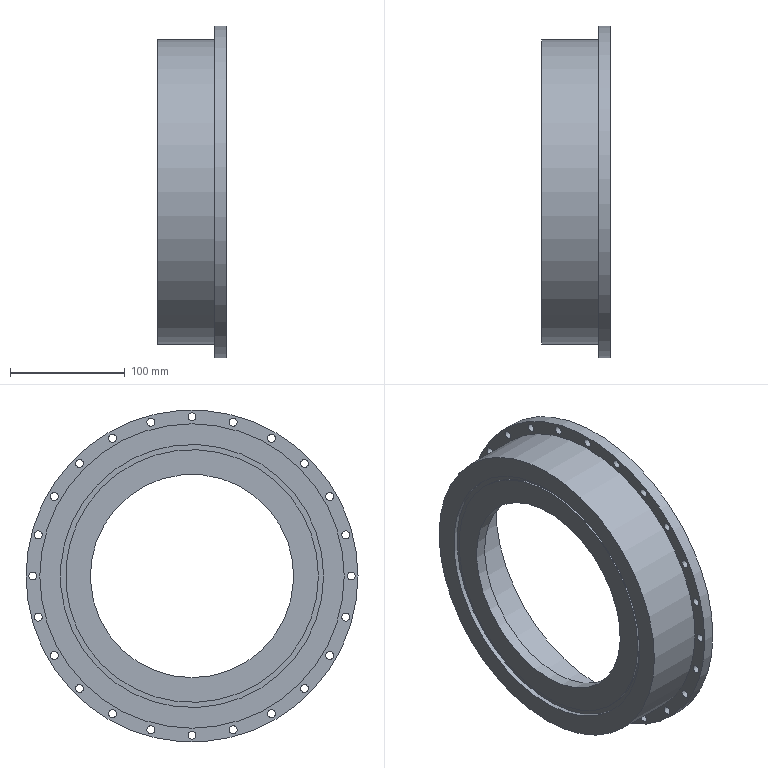Part | STEP file | Brake disc | 1 solid | 36 faces | box 60 x 289 x 289 mm | volume 806797 mm3 | cylinder 30 | plane 6 | commonest cylinder face diameters 7 x24 177 x1 220 x1 229 x1 245 x1 265 x1
STEP:
#1=CARTESIAN_POINT('',(-12.,0.,-132.5));
#2=VERTEX_POINT('',#1);
#3=CARTESIAN_POINT('',(-12.,0.,0.));
#4=DIRECTION('',(-1.,0.,0.));
#5=DIRECTION('',(0.,0.,-1.));
#6=AXIS2_PLACEMENT_3D('',#3,#4,#5);
#7=CIRCLE('',#6,132.5);
#8=EDGE_CURVE('',#2,#2,#7,.T.);
#9=ORIENTED_EDGE('',*,*,#8,.T.);
#10=EDGE_LOOP('',(#9));
#11=FACE_BOUND('',#10,.T.);
#12=CARTESIAN_POINT('',(-12.,-114.5,0.));
#13=VERTEX_POINT('',#12);
#14=CARTESIAN_POINT('',(-12.,0.,0.));
#15=DIRECTION('',(-1.,0.,0.));
#16=DIRECTION('',(0.,-1.,0.));
#17=AXIS2_PLACEMENT_3D('',#14,#15,#16);
#18=CIRCLE('',#17,114.5);
#19=EDGE_CURVE('',#13,#13,#18,.F.);
#20=ORIENTED_EDGE('',*,*,#19,.T.);
#21=EDGE_LOOP('',(#20));
#22=FACE_BOUND('',#21,.T.);
#23=CARTESIAN_POINT('',(-12.,0.,0.));
#24=DIRECTION('',(1.,0.,0.));
#25=DIRECTION('',(0.,1.,0.));
#26=AXIS2_PLACEMENT_3D('',#23,#24,#25);
#27=PLANE('',#26);
#28=ADVANCED_FACE('',(#11,#22),#27,.F.);
#29=CARTESIAN_POINT('',(-10.,-110.,0.));
#30=VERTEX_POINT('',#29);
#31=CARTESIAN_POINT('',(-10.,0.,0.));
#32=DIRECTION('',(-1.,0.,0.));
#33=DIRECTION('',(0.,-1.,0.));
#34=AXIS2_PLACEMENT_3D('',#31,#32,#33);
#35=CIRCLE('',#34,110.);
#36=EDGE_CURVE('',#30,#30,#35,.T.);
#37=ORIENTED_EDGE('',*,*,#36,.T.);
#38=EDGE_LOOP('',(#37));
#39=FACE_BOUND('',#38,.T.);
#40=CARTESIAN_POINT('',(-10.,0.,-88.5));
#41=VERTEX_POINT('',#40);
#42=CARTESIAN_POINT('',(-10.,0.,0.));
#43=DIRECTION('',(1.,0.,0.));
#44=DIRECTION('',(0.,0.,-1.));
#45=AXIS2_PLACEMENT_3D('',#42,#43,#44);
#46=CIRCLE('',#45,88.5);
#47=EDGE_CURVE('',#41,#41,#46,.T.);
#48=ORIENTED_EDGE('',*,*,#47,.T.);
#49=EDGE_LOOP('',(#48));
#50=FACE_BOUND('',#49,.T.);
#51=CARTESIAN_POINT('',(-10.,0.,0.));
#52=DIRECTION('',(1.,0.,0.));
#53=DIRECTION('',(0.,0.,-1.));
#54=AXIS2_PLACEMENT_3D('',#51,#52,#53);
#55=PLANE('',#54);
#56=ADVANCED_FACE('',(#39,#50),#55,.F.);
#57=CARTESIAN_POINT('',(-8.,-114.5,0.));
#58=VERTEX_POINT('',#57);
#59=CARTESIAN_POINT('',(-8.,0.,0.));
#60=DIRECTION('',(-1.,0.,0.));
#61=DIRECTION('',(0.,-1.,0.));
#62=AXIS2_PLACEMENT_3D('',#59,#60,#61);
#63=CIRCLE('',#62,114.5);
#64=EDGE_CURVE('',#58,#58,#63,.T.);
#65=ORIENTED_EDGE('',*,*,#64,.F.);
#66=EDGE_LOOP('',(#65));
#67=FACE_OUTER_BOUND('',#66,.T.);
#68=ORIENTED_EDGE('',*,*,#19,.F.);
#69=EDGE_LOOP('',(#68));
#70=FACE_OUTER_BOUND('',#69,.T.);
#71=CARTESIAN_POINT('',(-8.,0.,0.));
#72=DIRECTION('',(-1.,0.,0.));
#73=DIRECTION('',(0.,-1.,0.));
#74=AXIS2_PLACEMENT_3D('',#71,#72,#73);
#75=CYLINDRICAL_SURFACE('',#74,114.5);
#76=ADVANCED_FACE('',(#67,#70),#75,.F.);
#77=CARTESIAN_POINT('',(-8.,-110.,0.));
#78=VERTEX_POINT('',#77);
#79=CARTESIAN_POINT('',(-8.,0.,0.));
#80=DIRECTION('',(-1.,0.,0.));
#81=DIRECTION('',(0.,-1.,0.));
#82=AXIS2_PLACEMENT_3D('',#79,#80,#81);
#83=CIRCLE('',#82,110.);
#84=EDGE_CURVE('',#78,#78,#83,.T.);
#85=ORIENTED_EDGE('',*,*,#84,.T.);
#86=EDGE_LOOP('',(#85));
#87=FACE_OUTER_BOUND('',#86,.T.);
#88=ORIENTED_EDGE('',*,*,#36,.F.);
#89=EDGE_LOOP('',(#88));
#90=FACE_OUTER_BOUND('',#89,.T.);
#91=CARTESIAN_POINT('',(-8.,0.,0.));
#92=DIRECTION('',(-1.,0.,0.));
#93=DIRECTION('',(0.,-1.,0.));
#94=AXIS2_PLACEMENT_3D('',#91,#92,#93);
#95=CYLINDRICAL_SURFACE('',#94,110.);
#96=ADVANCED_FACE('',(#87,#90),#95,.T.);
#97=CARTESIAN_POINT('',(38.,0.,-132.5));
#98=VERTEX_POINT('',#97);
#99=CARTESIAN_POINT('',(38.,0.,0.));
#100=DIRECTION('',(-1.,0.,0.));
#101=DIRECTION('',(0.,0.,-1.));
#102=AXIS2_PLACEMENT_3D('',#99,#100,#101);
#103=CIRCLE('',#102,132.5);
#104=EDGE_CURVE('',#98,#98,#103,.F.);
#105=ORIENTED_EDGE('',*,*,#104,.F.);
#106=EDGE_LOOP('',(#105));
#107=FACE_OUTER_BOUND('',#106,.T.);
#108=ORIENTED_EDGE('',*,*,#8,.F.);
#109=EDGE_LOOP('',(#108));
#110=FACE_OUTER_BOUND('',#109,.T.);
#111=CARTESIAN_POINT('',(8.,0.,0.));
#112=DIRECTION('',(-1.,0.,0.));
#113=DIRECTION('',(0.,0.,-1.));
#114=AXIS2_PLACEMENT_3D('',#111,#112,#113);
#115=CYLINDRICAL_SURFACE('',#114,132.5);
#116=ADVANCED_FACE('',(#107,#110),#115,.T.);
#117=CARTESIAN_POINT('',(0.,0.,-88.5));
#118=VERTEX_POINT('',#117);
#119=CARTESIAN_POINT('',(0.,0.,0.));
#120=DIRECTION('',(1.,0.,0.));
#121=DIRECTION('',(0.,0.,-1.));
#122=AXIS2_PLACEMENT_3D('',#119,#120,#121);
#123=CIRCLE('',#122,88.5);
#124=EDGE_CURVE('',#118,#118,#123,.F.);
#125=ORIENTED_EDGE('',*,*,#124,.F.);
#126=EDGE_LOOP('',(#125));
#127=FACE_OUTER_BOUND('',#126,.T.);
#128=ORIENTED_EDGE('',*,*,#47,.F.);
#129=EDGE_LOOP('',(#128));
#130=FACE_OUTER_BOUND('',#129,.T.);
#131=CARTESIAN_POINT('',(-10.,0.,0.));
#132=DIRECTION('',(1.,0.,0.));
#133=DIRECTION('',(0.,0.,-1.));
#134=AXIS2_PLACEMENT_3D('',#131,#132,#133);
#135=CYLINDRICAL_SURFACE('',#134,88.5);
#136=ADVANCED_FACE('',(#127,#130),#135,.F.);
#137=ORIENTED_EDGE('',*,*,#64,.T.);
#138=EDGE_LOOP('',(#137));
#139=FACE_BOUND('',#138,.T.);
#140=ORIENTED_EDGE('',*,*,#84,.F.);
#141=EDGE_LOOP('',(#140));
#142=FACE_BOUND('',#141,.T.);
#143=CARTESIAN_POINT('',(-8.,0.,0.));
#144=DIRECTION('',(-1.,0.,0.));
#145=DIRECTION('',(0.,-1.,0.));
#146=AXIS2_PLACEMENT_3D('',#143,#144,#145);
#147=PLANE('',#146);
#148=ADVANCED_FACE('',(#139,#142),#147,.T.);
#149=CARTESIAN_POINT('',(38.,-144.5,0.));
#150=VERTEX_POINT('',#149);
#151=CARTESIAN_POINT('',(38.,0.,0.));
#152=DIRECTION('',(1.,0.,0.));
#153=DIRECTION('',(0.,-1.,0.));
#154=AXIS2_PLACEMENT_3D('',#151,#152,#153);
#155=CIRCLE('',#154,144.5);
#156=EDGE_CURVE('',#150,#150,#155,.T.);
#157=ORIENTED_EDGE('',*,*,#156,.F.);
#158=EDGE_LOOP('',(#157));
#159=FACE_BOUND('',#158,.T.);
#160=CARTESIAN_POINT('',(38.,137.161,36.752));
#161=VERTEX_POINT('',#160);
#162=CARTESIAN_POINT('',(38.,133.781,35.846));
#163=DIRECTION('',(1.,0.,0.));
#164=DIRECTION('',(0.,0.9659,0.2588));
#165=AXIS2_PLACEMENT_3D('',#162,#163,#164);
#166=CIRCLE('',#165,3.5);
#167=EDGE_CURVE('',#161,#161,#166,.T.);
#168=ORIENTED_EDGE('',*,*,#167,.T.);
#169=EDGE_LOOP('',(#168));
#170=FACE_BOUND('',#169,.T.);
#171=CARTESIAN_POINT('',(38.,122.976,71.));
#172=VERTEX_POINT('',#171);
#173=CARTESIAN_POINT('',(38.,119.945,69.25));
#174=DIRECTION('',(1.,0.,0.));
#175=DIRECTION('',(0.,0.866,0.5));
#176=AXIS2_PLACEMENT_3D('',#173,#174,#175);
#177=CIRCLE('',#176,3.5);
#178=EDGE_CURVE('',#172,#172,#177,.T.);
#179=ORIENTED_EDGE('',*,*,#178,.T.);
#180=EDGE_LOOP('',(#179));
#181=FACE_BOUND('',#180,.T.);
#182=CARTESIAN_POINT('',(38.,100.409,100.409));
#183=VERTEX_POINT('',#182);
#184=CARTESIAN_POINT('',(38.,97.934,97.934));
#185=DIRECTION('',(1.,0.,0.));
#186=DIRECTION('',(0.,0.7071,0.7071));
#187=AXIS2_PLACEMENT_3D('',#184,#185,#186);
#188=CIRCLE('',#187,3.5);
#189=EDGE_CURVE('',#183,#183,#188,.T.);
#190=ORIENTED_EDGE('',*,*,#189,.T.);
#191=EDGE_LOOP('',(#190));
#192=FACE_BOUND('',#191,.T.);
#193=CARTESIAN_POINT('',(38.,71.,122.976));
#194=VERTEX_POINT('',#193);
#195=CARTESIAN_POINT('',(38.,69.25,119.945));
#196=DIRECTION('',(1.,0.,0.));
#197=DIRECTION('',(0.,0.5,0.866));
#198=AXIS2_PLACEMENT_3D('',#195,#196,#197);
#199=CIRCLE('',#198,3.5);
#200=EDGE_CURVE('',#194,#194,#199,.T.);
#201=ORIENTED_EDGE('',*,*,#200,.T.);
#202=EDGE_LOOP('',(#201));
#203=FACE_BOUND('',#202,.T.);
#204=CARTESIAN_POINT('',(38.,36.752,137.161));
#205=VERTEX_POINT('',#204);
#206=CARTESIAN_POINT('',(38.,35.846,133.781));
#207=DIRECTION('',(1.,0.,0.));
#208=DIRECTION('',(0.,0.2588,0.9659));
#209=AXIS2_PLACEMENT_3D('',#206,#207,#208);
#210=CIRCLE('',#209,3.5);
#211=EDGE_CURVE('',#205,#205,#210,.T.);
#212=ORIENTED_EDGE('',*,*,#211,.T.);
#213=EDGE_LOOP('',(#212));
#214=FACE_BOUND('',#213,.T.);
#215=CARTESIAN_POINT('',(38.,0.,142.));
#216=VERTEX_POINT('',#215);
#217=CARTESIAN_POINT('',(38.,0.,138.5));
#218=DIRECTION('',(1.,0.,0.));
#219=DIRECTION('',(0.,0.,1.));
#220=AXIS2_PLACEMENT_3D('',#217,#218,#219);
#221=CIRCLE('',#220,3.5);
#222=EDGE_CURVE('',#216,#216,#221,.T.);
#223=ORIENTED_EDGE('',*,*,#222,.T.);
#224=EDGE_LOOP('',(#223));
#225=FACE_BOUND('',#224,.T.);
#226=CARTESIAN_POINT('',(38.,-36.752,137.161));
#227=VERTEX_POINT('',#226);
#228=CARTESIAN_POINT('',(38.,-35.846,133.781));
#229=DIRECTION('',(1.,0.,0.));
#230=DIRECTION('',(0.,-0.2588,0.9659));
#231=AXIS2_PLACEMENT_3D('',#228,#229,#230);
#232=CIRCLE('',#231,3.5);
#233=EDGE_CURVE('',#227,#227,#232,.T.);
#234=ORIENTED_EDGE('',*,*,#233,.T.);
#235=EDGE_LOOP('',(#234));
#236=FACE_BOUND('',#235,.T.);
#237=CARTESIAN_POINT('',(38.,-71.,122.976));
#238=VERTEX_POINT('',#237);
#239=CARTESIAN_POINT('',(38.,-69.25,119.945));
#240=DIRECTION('',(1.,0.,0.));
#241=DIRECTION('',(0.,-0.5,0.866));
#242=AXIS2_PLACEMENT_3D('',#239,#240,#241);
#243=CIRCLE('',#242,3.5);
#244=EDGE_CURVE('',#238,#238,#243,.T.);
#245=ORIENTED_EDGE('',*,*,#244,.T.);
#246=EDGE_LOOP('',(#245));
#247=FACE_BOUND('',#246,.T.);
#248=CARTESIAN_POINT('',(38.,-100.409,100.409));
#249=VERTEX_POINT('',#248);
#250=CARTESIAN_POINT('',(38.,-97.934,97.934));
#251=DIRECTION('',(1.,0.,0.));
#252=DIRECTION('',(0.,-0.7071,0.7071));
#253=AXIS2_PLACEMENT_3D('',#250,#251,#252);
#254=CIRCLE('',#253,3.5);
#255=EDGE_CURVE('',#249,#249,#254,.T.);
#256=ORIENTED_EDGE('',*,*,#255,.T.);
#257=EDGE_LOOP('',(#256));
#258=FACE_BOUND('',#257,.T.);
#259=CARTESIAN_POINT('',(38.,-122.976,71.));
#260=VERTEX_POINT('',#259);
#261=CARTESIAN_POINT('',(38.,-119.945,69.25));
#262=DIRECTION('',(1.,0.,0.));
#263=DIRECTION('',(0.,-0.866,0.5));
#264=AXIS2_PLACEMENT_3D('',#261,#262,#263);
#265=CIRCLE('',#264,3.5);
#266=EDGE_CURVE('',#260,#260,#265,.T.);
#267=ORIENTED_EDGE('',*,*,#266,.T.);
#268=EDGE_LOOP('',(#267));
#269=FACE_BOUND('',#268,.T.);
#270=CARTESIAN_POINT('',(38.,-137.161,36.752));
#271=VERTEX_POINT('',#270);
#272=CARTESIAN_POINT('',(38.,-133.781,35.846));
#273=DIRECTION('',(1.,0.,0.));
#274=DIRECTION('',(0.,-0.9659,0.2588));
#275=AXIS2_PLACEMENT_3D('',#272,#273,#274);
#276=CIRCLE('',#275,3.5);
#277=EDGE_CURVE('',#271,#271,#276,.T.);
#278=ORIENTED_EDGE('',*,*,#277,.T.);
#279=EDGE_LOOP('',(#278));
#280=FACE_BOUND('',#279,.T.);
#281=CARTESIAN_POINT('',(38.,-142.,0.));
#282=VERTEX_POINT('',#281);
#283=CARTESIAN_POINT('',(38.,-138.5,0.));
#284=DIRECTION('',(1.,0.,0.));
#285=DIRECTION('',(0.,-1.,0.));
#286=AXIS2_PLACEMENT_3D('',#283,#284,#285);
#287=CIRCLE('',#286,3.5);
#288=EDGE_CURVE('',#282,#282,#287,.T.);
#289=ORIENTED_EDGE('',*,*,#288,.T.);
#290=EDGE_LOOP('',(#289));
#291=FACE_BOUND('',#290,.T.);
#292=CARTESIAN_POINT('',(38.,-137.161,-36.752));
#293=VERTEX_POINT('',#292);
#294=CARTESIAN_POINT('',(38.,-133.781,-35.846));
#295=DIRECTION('',(1.,0.,0.));
#296=DIRECTION('',(0.,-0.9659,-0.2588));
#297=AXIS2_PLACEMENT_3D('',#294,#295,#296);
#298=CIRCLE('',#297,3.5);
#299=EDGE_CURVE('',#293,#293,#298,.T.);
#300=ORIENTED_EDGE('',*,*,#299,.T.);
#301=EDGE_LOOP('',(#300));
#302=FACE_BOUND('',#301,.T.);
#303=CARTESIAN_POINT('',(38.,-122.976,-71.));
#304=VERTEX_POINT('',#303);
#305=CARTESIAN_POINT('',(38.,-119.945,-69.25));
#306=DIRECTION('',(1.,0.,0.));
#307=DIRECTION('',(0.,-0.866,-0.5));
#308=AXIS2_PLACEMENT_3D('',#305,#306,#307);
#309=CIRCLE('',#308,3.5);
#310=EDGE_CURVE('',#304,#304,#309,.T.);
#311=ORIENTED_EDGE('',*,*,#310,.T.);
#312=EDGE_LOOP('',(#311));
#313=FACE_BOUND('',#312,.T.);
#314=CARTESIAN_POINT('',(38.,-100.409,-100.409));
#315=VERTEX_POINT('',#314);
#316=CARTESIAN_POINT('',(38.,-97.934,-97.934));
#317=DIRECTION('',(1.,0.,0.));
#318=DIRECTION('',(0.,-0.7071,-0.7071));
#319=AXIS2_PLACEMENT_3D('',#316,#317,#318);
#320=CIRCLE('',#319,3.5);
#321=EDGE_CURVE('',#315,#315,#320,.T.);
#322=ORIENTED_EDGE('',*,*,#321,.T.);
#323=EDGE_LOOP('',(#322));
#324=FACE_BOUND('',#323,.T.);
#325=CARTESIAN_POINT('',(38.,-71.,-122.976));
#326=VERTEX_POINT('',#325);
#327=CARTESIAN_POINT('',(38.,-69.25,-119.945));
#328=DIRECTION('',(1.,0.,0.));
#329=DIRECTION('',(0.,-0.5,-0.866));
#330=AXIS2_PLACEMENT_3D('',#327,#328,#329);
#331=CIRCLE('',#330,3.5);
#332=EDGE_CURVE('',#326,#326,#331,.T.);
#333=ORIENTED_EDGE('',*,*,#332,.T.);
#334=EDGE_LOOP('',(#333));
#335=FACE_BOUND('',#334,.T.);
#336=CARTESIAN_POINT('',(38.,-36.752,-137.161));
#337=VERTEX_POINT('',#336);
#338=CARTESIAN_POINT('',(38.,-35.846,-133.781));
#339=DIRECTION('',(1.,0.,0.));
#340=DIRECTION('',(0.,-0.2588,-0.9659));
#341=AXIS2_PLACEMENT_3D('',#338,#339,#340);
#342=CIRCLE('',#341,3.5);
#343=EDGE_CURVE('',#337,#337,#342,.T.);
#344=ORIENTED_EDGE('',*,*,#343,.T.);
#345=EDGE_LOOP('',(#344));
#346=FACE_BOUND('',#345,.T.);
#347=CARTESIAN_POINT('',(38.,0.,-142.));
#348=VERTEX_POINT('',#347);
#349=CARTESIAN_POINT('',(38.,0.,-138.5));
#350=DIRECTION('',(1.,0.,0.));
#351=DIRECTION('',(0.,0.,-1.));
#352=AXIS2_PLACEMENT_3D('',#349,#350,#351);
#353=CIRCLE('',#352,3.5);
#354=EDGE_CURVE('',#348,#348,#353,.T.);
#355=ORIENTED_EDGE('',*,*,#354,.T.);
#356=EDGE_LOOP('',(#355));
#357=FACE_BOUND('',#356,.T.);
#358=CARTESIAN_POINT('',(38.,36.752,-137.161));
#359=VERTEX_POINT('',#358);
#360=CARTESIAN_POINT('',(38.,35.846,-133.781));
#361=DIRECTION('',(1.,0.,0.));
#362=DIRECTION('',(0.,0.2588,-0.9659));
#363=AXIS2_PLACEMENT_3D('',#360,#361,#362);
#364=CIRCLE('',#363,3.5);
#365=EDGE_CURVE('',#359,#359,#364,.T.);
#366=ORIENTED_EDGE('',*,*,#365,.T.);
#367=EDGE_LOOP('',(#366));
#368=FACE_BOUND('',#367,.T.);
#369=CARTESIAN_POINT('',(38.,71.,-122.976));
#370=VERTEX_POINT('',#369);
#371=CARTESIAN_POINT('',(38.,69.25,-119.945));
#372=DIRECTION('',(1.,0.,0.));
#373=DIRECTION('',(0.,0.5,-0.866));
#374=AXIS2_PLACEMENT_3D('',#371,#372,#373);
#375=CIRCLE('',#374,3.5);
#376=EDGE_CURVE('',#370,#370,#375,.T.);
#377=ORIENTED_EDGE('',*,*,#376,.T.);
#378=EDGE_LOOP('',(#377));
#379=FACE_BOUND('',#378,.T.);
#380=CARTESIAN_POINT('',(38.,100.409,-100.409));
#381=VERTEX_POINT('',#380);
#382=CARTESIAN_POINT('',(38.,97.934,-97.934));
#383=DIRECTION('',(1.,0.,0.));
#384=DIRECTION('',(0.,0.7071,-0.7071));
#385=AXIS2_PLACEMENT_3D('',#382,#383,#384);
#386=CIRCLE('',#385,3.5);
#387=EDGE_CURVE('',#381,#381,#386,.T.);
#388=ORIENTED_EDGE('',*,*,#387,.T.);
#389=EDGE_LOOP('',(#388));
#390=FACE_BOUND('',#389,.T.);
#391=CARTESIAN_POINT('',(38.,122.976,-71.));
#392=VERTEX_POINT('',#391);
#393=CARTESIAN_POINT('',(38.,119.945,-69.25));
#394=DIRECTION('',(1.,0.,0.));
#395=DIRECTION('',(0.,0.866,-0.5));
#396=AXIS2_PLACEMENT_3D('',#393,#394,#395);
#397=CIRCLE('',#396,3.5);
#398=EDGE_CURVE('',#392,#392,#397,.T.);
#399=ORIENTED_EDGE('',*,*,#398,.T.);
#400=EDGE_LOOP('',(#399));
#401=FACE_BOUND('',#400,.T.);
#402=CARTESIAN_POINT('',(38.,137.161,-36.752));
#403=VERTEX_POINT('',#402);
#404=CARTESIAN_POINT('',(38.,133.781,-35.846));
#405=DIRECTION('',(1.,0.,0.));
#406=DIRECTION('',(0.,0.9659,-0.2588));
#407=AXIS2_PLACEMENT_3D('',#404,#405,#406);
#408=CIRCLE('',#407,3.5);
#409=EDGE_CURVE('',#403,#403,#408,.T.);
#410=ORIENTED_EDGE('',*,*,#409,.T.);
#411=EDGE_LOOP('',(#410));
#412=FACE_BOUND('',#411,.T.);
#413=ORIENTED_EDGE('',*,*,#104,.T.);
#414=EDGE_LOOP('',(#413));
#415=FACE_BOUND('',#414,.T.);
#416=CARTESIAN_POINT('',(38.,142.,0.));
#417=VERTEX_POINT('',#416);
#418=CARTESIAN_POINT('',(38.,138.5,0.));
#419=DIRECTION('',(1.,0.,0.));
#420=DIRECTION('',(0.,1.,0.));
#421=AXIS2_PLACEMENT_3D('',#418,#419,#420);
#422=CIRCLE('',#421,3.5);
#423=EDGE_CURVE('',#417,#417,#422,.T.);
#424=ORIENTED_EDGE('',*,*,#423,.T.);
#425=EDGE_LOOP('',(#424));
#426=FACE_BOUND('',#425,.T.);
#427=CARTESIAN_POINT('',(38.,0.,0.));
#428=DIRECTION('',(1.,0.,0.));
#429=DIRECTION('',(0.,-1.,0.));
#430=AXIS2_PLACEMENT_3D('',#427,#428,#429);
#431=PLANE('',#430);
#432=ADVANCED_FACE('',(#159,#170,#181,#192,#203,#214,#225,#236,#247,#258,#269,#280,#291,#302,#313,#324,#335,#346,#357,#368,#379,#390,#401,#412,#415,#426),#431,.F.);
#433=CARTESIAN_POINT('',(0.,0.,-122.5));
#434=VERTEX_POINT('',#433);
#435=CARTESIAN_POINT('',(0.,0.,0.));
#436=DIRECTION('',(1.,0.,0.));
#437=DIRECTION('',(0.,0.,-1.));
#438=AXIS2_PLACEMENT_3D('',#435,#436,#437);
#439=CIRCLE('',#438,122.5);
#440=EDGE_CURVE('',#434,#434,#439,.F.);
#441=ORIENTED_EDGE('',*,*,#440,.F.);
#442=EDGE_LOOP('',(#441));
#443=FACE_BOUND('',#442,.T.);
#444=ORIENTED_EDGE('',*,*,#124,.T.);
#445=EDGE_LOOP('',(#444));
#446=FACE_BOUND('',#445,.T.);
#447=CARTESIAN_POINT('',(0.,0.,0.));
#448=DIRECTION('',(1.,0.,0.));
#449=DIRECTION('',(0.,0.,-1.));
#450=AXIS2_PLACEMENT_3D('',#447,#448,#449);
#451=PLANE('',#450);
#452=ADVANCED_FACE('',(#443,#446),#451,.T.);
#453=CARTESIAN_POINT('',(48.,-144.5,0.));
#454=VERTEX_POINT('',#453);
#455=CARTESIAN_POINT('',(48.,0.,0.));
#456=DIRECTION('',(1.,0.,0.));
#457=DIRECTION('',(0.,-1.,0.));
#458=AXIS2_PLACEMENT_3D('',#455,#456,#457);
#459=CIRCLE('',#458,144.5);
#460=EDGE_CURVE('',#454,#454,#459,.T.);
#461=ORIENTED_EDGE('',*,*,#460,.F.);
#462=EDGE_LOOP('',(#461));
#463=FACE_OUTER_BOUND('',#462,.T.);
#464=ORIENTED_EDGE('',*,*,#156,.T.);
#465=EDGE_LOOP('',(#464));
#466=FACE_OUTER_BOUND('',#465,.T.);
#467=CARTESIAN_POINT('',(38.,0.,0.));
#468=DIRECTION('',(1.,0.,0.));
#469=DIRECTION('',(0.,-1.,0.));
#470=AXIS2_PLACEMENT_3D('',#467,#468,#469);
#471=CYLINDRICAL_SURFACE('',#470,144.5);
#472=ADVANCED_FACE('',(#463,#466),#471,.T.);
#473=CARTESIAN_POINT('',(48.,137.161,36.752));
#474=VERTEX_POINT('',#473);
#475=CARTESIAN_POINT('',(48.,133.781,35.846));
#476=DIRECTION('',(1.,0.,0.));
#477=DIRECTION('',(0.,0.9659,0.2588));
#478=AXIS2_PLACEMENT_3D('',#475,#476,#477);
#479=CIRCLE('',#478,3.5);
#480=EDGE_CURVE('',#474,#474,#479,.F.);
#481=ORIENTED_EDGE('',*,*,#480,.F.);
#482=EDGE_LOOP('',(#481));
#483=FACE_OUTER_BOUND('',#482,.T.);
#484=ORIENTED_EDGE('',*,*,#167,.F.);
#485=EDGE_LOOP('',(#484));
#486=FACE_OUTER_BOUND('',#485,.T.);
#487=CARTESIAN_POINT('',(8.,133.781,35.846));
#488=DIRECTION('',(1.,0.,0.));
#489=DIRECTION('',(0.,0.9659,0.2588));
#490=AXIS2_PLACEMENT_3D('',#487,#488,#489);
#491=CYLINDRICAL_SURFACE('',#490,3.5);
#492=ADVANCED_FACE('',(#483,#486),#491,.F.);
#493=CARTESIAN_POINT('',(48.,122.976,71.));
#494=VERTEX_POINT('',#493);
#495=CARTESIAN_POINT('',(48.,119.945,69.25));
#496=DIRECTION('',(1.,0.,0.));
#497=DIRECTION('',(0.,0.866,0.5));
#498=AXIS2_PLACEMENT_3D('',#495,#496,#497);
#499=CIRCLE('',#498,3.5);
#500=EDGE_CURVE('',#494,#494,#499,.F.);
#501=ORIENTED_EDGE('',*,*,#500,.F.);
#502=EDGE_LOOP('',(#501));
#503=FACE_OUTER_BOUND('',#502,.T.);
#504=ORIENTED_EDGE('',*,*,#178,.F.);
#505=EDGE_LOOP('',(#504));
#506=FACE_OUTER_BOUND('',#505,.T.);
#507=CARTESIAN_POINT('',(8.,119.945,69.25));
#508=DIRECTION('',(1.,0.,0.));
#509=DIRECTION('',(0.,0.866,0.5));
#510=AXIS2_PLACEMENT_3D('',#507,#508,#509);
#511=CYLINDRICAL_SURFACE('',#510,3.5);
#512=ADVANCED_FACE('',(#503,#506),#511,.F.);
#513=CARTESIAN_POINT('',(48.,100.409,100.409));
#514=VERTEX_POINT('',#513);
#515=CARTESIAN_POINT('',(48.,97.934,97.934));
#516=DIRECTION('',(1.,0.,0.));
#517=DIRECTION('',(0.,0.7071,0.7071));
#518=AXIS2_PLACEMENT_3D('',#515,#516,#517);
#519=CIRCLE('',#518,3.5);
#520=EDGE_CURVE('',#514,#514,#519,.F.);
#521=ORIENTED_EDGE('',*,*,#520,.F.);
#522=EDGE_LOOP('',(#521));
#523=FACE_OUTER_BOUND('',#522,.T.);
#524=ORIENTED_EDGE('',*,*,#189,.F.);
#525=EDGE_LOOP('',(#524));
#526=FACE_OUTER_BOUND('',#525,.T.);
#527=CARTESIAN_POINT('',(8.,97.934,97.934));
#528=DIRECTION('',(1.,0.,0.));
#529=DIRECTION('',(0.,0.7071,0.7071));
#530=AXIS2_PLACEMENT_3D('',#527,#528,#529);
#531=CYLINDRICAL_SURFACE('',#530,3.5);
#532=ADVANCED_FACE('',(#523,#526),#531,.F.);
#533=CARTESIAN_POINT('',(48.,71.,122.976));
#534=VERTEX_POINT('',#533);
#535=CARTESIAN_POINT('',(48.,69.25,119.945));
#536=DIRECTION('',(1.,0.,0.));
#537=DIRECTION('',(0.,0.5,0.866));
#538=AXIS2_PLACEMENT_3D('',#535,#536,#537);
#539=CIRCLE('',#538,3.5);
#540=EDGE_CURVE('',#534,#534,#539,.F.);
#541=ORIENTED_EDGE('',*,*,#540,.F.);
#542=EDGE_LOOP('',(#541));
#543=FACE_OUTER_BOUND('',#542,.T.);
#544=ORIENTED_EDGE('',*,*,#200,.F.);
#545=EDGE_LOOP('',(#544));
#546=FACE_OUTER_BOUND('',#545,.T.);
#547=CARTESIAN_POINT('',(8.,69.25,119.945));
#548=DIRECTION('',(1.,0.,0.));
#549=DIRECTION('',(0.,0.5,0.866));
#550=AXIS2_PLACEMENT_3D('',#547,#548,#549);
#551=CYLINDRICAL_SURFACE('',#550,3.5);
#552=ADVANCED_FACE('',(#543,#546),#551,.F.);
#553=CARTESIAN_POINT('',(48.,36.752,137.161));
#554=VERTEX_POINT('',#553);
#555=CARTESIAN_POINT('',(48.,35.846,133.781));
#556=DIRECTION('',(1.,0.,0.));
#557=DIRECTION('',(0.,0.2588,0.9659));
#558=AXIS2_PLACEMENT_3D('',#555,#556,#557);
#559=CIRCLE('',#558,3.5);
#560=EDGE_CURVE('',#554,#554,#559,.F.);
#561=ORIENTED_EDGE('',*,*,#560,.F.);
#562=EDGE_LOOP('',(#561));
#563=FACE_OUTER_BOUND('',#562,.T.);
#564=ORIENTED_EDGE('',*,*,#211,.F.);
#565=EDGE_LOOP('',(#564));
#566=FACE_OUTER_BOUND('',#565,.T.);
#567=CARTESIAN_POINT('',(8.,35.846,133.781));
#568=DIRECTION('',(1.,0.,0.));
#569=DIRECTION('',(0.,0.2588,0.9659));
#570=AXIS2_PLACEMENT_3D('',#567,#568,#569);
#571=CYLINDRICAL_SURFACE('',#570,3.5);
#572=ADVANCED_FACE('',(#563,#566),#571,.F.);
#573=CARTESIAN_POINT('',(48.,0.,142.));
#574=VERTEX_POINT('',#573);
#575=CARTESIAN_POINT('',(48.,0.,138.5));
#576=DIRECTION('',(1.,0.,0.));
#577=DIRECTION('',(0.,0.,1.));
#578=AXIS2_PLACEMENT_3D('',#575,#576,#577);
#579=CIRCLE('',#578,3.5);
#580=EDGE_CURVE('',#574,#574,#579,.F.);
#581=ORIENTED_EDGE('',*,*,#580,.F.);
#582=EDGE_LOOP('',(#581));
#583=FACE_OUTER_BOUND('',#582,.T.);
#584=ORIENTED_EDGE('',*,*,#222,.F.);
#585=EDGE_LOOP('',(#584));
#586=FACE_OUTER_BOUND('',#585,.T.);
#587=CARTESIAN_POINT('',(8.,0.,138.5));
#588=DIRECTION('',(1.,0.,0.));
#589=DIRECTION('',(0.,0.,1.));
#590=AXIS2_PLACEMENT_3D('',#587,#588,#589);
#591=CYLINDRICAL_SURFACE('',#590,3.5);
#592=ADVANCED_FACE('',(#583,#586),#591,.F.);
#593=CARTESIAN_POINT('',(48.,-36.752,137.161));
#594=VERTEX_POINT('',#593);
#595=CARTESIAN_POINT('',(48.,-35.846,133.781));
#596=DIRECTION('',(1.,0.,0.));
#597=DIRECTION('',(0.,-0.2588,0.9659));
#598=AXIS2_PLACEMENT_3D('',#595,#596,#597);
#599=CIRCLE('',#598,3.5);
#600=EDGE_CURVE('',#594,#594,#599,.F.);
#601=ORIENTED_EDGE('',*,*,#600,.F.);
#602=EDGE_LOOP('',(#601));
#603=FACE_OUTER_BOUND('',#602,.T.);
#604=ORIENTED_EDGE('',*,*,#233,.F.);
#605=EDGE_LOOP('',(#604));
#606=FACE_OUTER_BOUND('',#605,.T.);
#607=CARTESIAN_POINT('',(8.,-35.846,133.781));
#608=DIRECTION('',(1.,0.,0.));
#609=DIRECTION('',(0.,-0.2588,0.9659));
#610=AXIS2_PLACEMENT_3D('',#607,#608,#609);
#611=CYLINDRICAL_SURFACE('',#610,3.5);
#612=ADVANCED_FACE('',(#603,#606),#611,.F.);
#613=CARTESIAN_POINT('',(48.,-71.,122.976));
#614=VERTEX_POINT('',#613);
#615=CARTESIAN_POINT('',(48.,-69.25,119.945));
#616=DIRECTION('',(1.,0.,0.));
#617=DIRECTION('',(0.,-0.5,0.866));
#618=AXIS2_PLACEMENT_3D('',#615,#616,#617);
#619=CIRCLE('',#618,3.5);
#620=EDGE_CURVE('',#614,#614,#619,.F.);
#621=ORIENTED_EDGE('',*,*,#620,.F.);
#622=EDGE_LOOP('',(#621));
#623=FACE_OUTER_BOUND('',#622,.T.);
#624=ORIENTED_EDGE('',*,*,#244,.F.);
#625=EDGE_LOOP('',(#624));
#626=FACE_OUTER_BOUND('',#625,.T.);
#627=CARTESIAN_POINT('',(8.,-69.25,119.945));
#628=DIRECTION('',(1.,0.,0.));
#629=DIRECTION('',(0.,-0.5,0.866));
#630=AXIS2_PLACEMENT_3D('',#627,#628,#629);
#631=CYLINDRICAL_SURFACE('',#630,3.5);
#632=ADVANCED_FACE('',(#623,#626),#631,.F.);
#633=CARTESIAN_POINT('',(48.,-100.409,100.409));
#634=VERTEX_POINT('',#633);
#635=CARTESIAN_POINT('',(48.,-97.934,97.934));
#636=DIRECTION('',(1.,0.,0.));
#637=DIRECTION('',(0.,-0.7071,0.7071));
#638=AXIS2_PLACEMENT_3D('',#635,#636,#637);
#639=CIRCLE('',#638,3.5);
#640=EDGE_CURVE('',#634,#634,#639,.F.);
#641=ORIENTED_EDGE('',*,*,#640,.F.);
#642=EDGE_LOOP('',(#641));
#643=FACE_OUTER_BOUND('',#642,.T.);
#644=ORIENTED_EDGE('',*,*,#255,.F.);
#645=EDGE_LOOP('',(#644));
#646=FACE_OUTER_BOUND('',#645,.T.);
#647=CARTESIAN_POINT('',(8.,-97.934,97.934));
#648=DIRECTION('',(1.,0.,0.));
#649=DIRECTION('',(0.,-0.7071,0.7071));
#650=AXIS2_PLACEMENT_3D('',#647,#648,#649);
#651=CYLINDRICAL_SURFACE('',#650,3.5);
#652=ADVANCED_FACE('',(#643,#646),#651,.F.);
#653=CARTESIAN_POINT('',(48.,-122.976,71.));
#654=VERTEX_POINT('',#653);
#655=CARTESIAN_POINT('',(48.,-119.945,69.25));
#656=DIRECTION('',(1.,0.,0.));
#657=DIRECTION('',(0.,-0.866,0.5));
#658=AXIS2_PLACEMENT_3D('',#655,#656,#657);
#659=CIRCLE('',#658,3.5);
#660=EDGE_CURVE('',#654,#654,#659,.F.);
#661=ORIENTED_EDGE('',*,*,#660,.F.);
#662=EDGE_LOOP('',(#661));
#663=FACE_OUTER_BOUND('',#662,.T.);
#664=ORIENTED_EDGE('',*,*,#266,.F.);
#665=EDGE_LOOP('',(#664));
#666=FACE_OUTER_BOUND('',#665,.T.);
#667=CARTESIAN_POINT('',(8.,-119.945,69.25));
#668=DIRECTION('',(1.,0.,0.));
#669=DIRECTION('',(0.,-0.866,0.5));
#670=AXIS2_PLACEMENT_3D('',#667,#668,#669);
#671=CYLINDRICAL_SURFACE('',#670,3.5);
#672=ADVANCED_FACE('',(#663,#666),#671,.F.);
#673=CARTESIAN_POINT('',(48.,-137.161,36.752));
#674=VERTEX_POINT('',#673);
#675=CARTESIAN_POINT('',(48.,-133.781,35.846));
#676=DIRECTION('',(1.,0.,0.));
#677=DIRECTION('',(0.,-0.9659,0.2588));
#678=AXIS2_PLACEMENT_3D('',#675,#676,#677);
#679=CIRCLE('',#678,3.5);
#680=EDGE_CURVE('',#674,#674,#679,.F.);
#681=ORIENTED_EDGE('',*,*,#680,.F.);
#682=EDGE_LOOP('',(#681));
#683=FACE_OUTER_BOUND('',#682,.T.);
#684=ORIENTED_EDGE('',*,*,#277,.F.);
#685=EDGE_LOOP('',(#684));
#686=FACE_OUTER_BOUND('',#685,.T.);
#687=CARTESIAN_POINT('',(8.,-133.781,35.846));
#688=DIRECTION('',(1.,0.,0.));
#689=DIRECTION('',(0.,-0.9659,0.2588));
#690=AXIS2_PLACEMENT_3D('',#687,#688,#689);
#691=CYLINDRICAL_SURFACE('',#690,3.5);
#692=ADVANCED_FACE('',(#683,#686),#691,.F.);
#693=CARTESIAN_POINT('',(48.,-142.,0.));
#694=VERTEX_POINT('',#693);
#695=CARTESIAN_POINT('',(48.,-138.5,0.));
#696=DIRECTION('',(1.,0.,0.));
#697=DIRECTION('',(0.,-1.,0.));
#698=AXIS2_PLACEMENT_3D('',#695,#696,#697);
#699=CIRCLE('',#698,3.5);
#700=EDGE_CURVE('',#694,#694,#699,.F.);
#701=ORIENTED_EDGE('',*,*,#700,.F.);
#702=EDGE_LOOP('',(#701));
#703=FACE_OUTER_BOUND('',#702,.T.);
#704=ORIENTED_EDGE('',*,*,#288,.F.);
#705=EDGE_LOOP('',(#704));
#706=FACE_OUTER_BOUND('',#705,.T.);
#707=CARTESIAN_POINT('',(8.,-138.5,0.));
#708=DIRECTION('',(1.,0.,0.));
#709=DIRECTION('',(0.,-1.,0.));
#710=AXIS2_PLACEMENT_3D('',#707,#708,#709);
#711=CYLINDRICAL_SURFACE('',#710,3.5);
#712=ADVANCED_FACE('',(#703,#706),#711,.F.);
#713=CARTESIAN_POINT('',(48.,-137.161,-36.752));
#714=VERTEX_POINT('',#713);
#715=CARTESIAN_POINT('',(48.,-133.781,-35.846));
#716=DIRECTION('',(1.,0.,0.));
#717=DIRECTION('',(0.,-0.9659,-0.2588));
#718=AXIS2_PLACEMENT_3D('',#715,#716,#717);
#719=CIRCLE('',#718,3.5);
#720=EDGE_CURVE('',#714,#714,#719,.F.);
#721=ORIENTED_EDGE('',*,*,#720,.F.);
#722=EDGE_LOOP('',(#721));
#723=FACE_OUTER_BOUND('',#722,.T.);
#724=ORIENTED_EDGE('',*,*,#299,.F.);
#725=EDGE_LOOP('',(#724));
#726=FACE_OUTER_BOUND('',#725,.T.);
#727=CARTESIAN_POINT('',(8.,-133.781,-35.846));
#728=DIRECTION('',(1.,0.,0.));
#729=DIRECTION('',(0.,-0.9659,-0.2588));
#730=AXIS2_PLACEMENT_3D('',#727,#728,#729);
#731=CYLINDRICAL_SURFACE('',#730,3.5);
#732=ADVANCED_FACE('',(#723,#726),#731,.F.);
#733=CARTESIAN_POINT('',(48.,-122.976,-71.));
#734=VERTEX_POINT('',#733);
#735=CARTESIAN_POINT('',(48.,-119.945,-69.25));
#736=DIRECTION('',(1.,0.,0.));
#737=DIRECTION('',(0.,-0.866,-0.5));
#738=AXIS2_PLACEMENT_3D('',#735,#736,#737);
#739=CIRCLE('',#738,3.5);
#740=EDGE_CURVE('',#734,#734,#739,.F.);
#741=ORIENTED_EDGE('',*,*,#740,.F.);
#742=EDGE_LOOP('',(#741));
#743=FACE_OUTER_BOUND('',#742,.T.);
#744=ORIENTED_EDGE('',*,*,#310,.F.);
#745=EDGE_LOOP('',(#744));
#746=FACE_OUTER_BOUND('',#745,.T.);
#747=CARTESIAN_POINT('',(8.,-119.945,-69.25));
#748=DIRECTION('',(1.,0.,0.));
#749=DIRECTION('',(0.,-0.866,-0.5));
#750=AXIS2_PLACEMENT_3D('',#747,#748,#749);
#751=CYLINDRICAL_SURFACE('',#750,3.5);
#752=ADVANCED_FACE('',(#743,#746),#751,.F.);
#753=CARTESIAN_POINT('',(48.,-100.409,-100.409));
#754=VERTEX_POINT('',#753);
#755=CARTESIAN_POINT('',(48.,-97.934,-97.934));
#756=DIRECTION('',(1.,0.,0.));
#757=DIRECTION('',(0.,-0.7071,-0.7071));
#758=AXIS2_PLACEMENT_3D('',#755,#756,#757);
#759=CIRCLE('',#758,3.5);
#760=EDGE_CURVE('',#754,#754,#759,.F.);
#761=ORIENTED_EDGE('',*,*,#760,.F.);
#762=EDGE_LOOP('',(#761));
#763=FACE_OUTER_BOUND('',#762,.T.);
#764=ORIENTED_EDGE('',*,*,#321,.F.);
#765=EDGE_LOOP('',(#764));
#766=FACE_OUTER_BOUND('',#765,.T.);
#767=CARTESIAN_POINT('',(8.,-97.934,-97.934));
#768=DIRECTION('',(1.,0.,0.));
#769=DIRECTION('',(0.,-0.7071,-0.7071));
#770=AXIS2_PLACEMENT_3D('',#767,#768,#769);
#771=CYLINDRICAL_SURFACE('',#770,3.5);
#772=ADVANCED_FACE('',(#763,#766),#771,.F.);
#773=CARTESIAN_POINT('',(48.,-71.,-122.976));
#774=VERTEX_POINT('',#773);
#775=CARTESIAN_POINT('',(48.,-69.25,-119.945));
#776=DIRECTION('',(1.,0.,0.));
#777=DIRECTION('',(0.,-0.5,-0.866));
#778=AXIS2_PLACEMENT_3D('',#775,#776,#777);
#779=CIRCLE('',#778,3.5);
#780=EDGE_CURVE('',#774,#774,#779,.F.);
#781=ORIENTED_EDGE('',*,*,#780,.F.);
#782=EDGE_LOOP('',(#781));
#783=FACE_OUTER_BOUND('',#782,.T.);
#784=ORIENTED_EDGE('',*,*,#332,.F.);
#785=EDGE_LOOP('',(#784));
#786=FACE_OUTER_BOUND('',#785,.T.);
#787=CARTESIAN_POINT('',(8.,-69.25,-119.945));
#788=DIRECTION('',(1.,0.,0.));
#789=DIRECTION('',(0.,-0.5,-0.866));
#790=AXIS2_PLACEMENT_3D('',#787,#788,#789);
#791=CYLINDRICAL_SURFACE('',#790,3.5);
#792=ADVANCED_FACE('',(#783,#786),#791,.F.);
#793=CARTESIAN_POINT('',(48.,-36.752,-137.161));
#794=VERTEX_POINT('',#793);
#795=CARTESIAN_POINT('',(48.,-35.846,-133.781));
#796=DIRECTION('',(1.,0.,0.));
#797=DIRECTION('',(0.,-0.2588,-0.9659));
#798=AXIS2_PLACEMENT_3D('',#795,#796,#797);
#799=CIRCLE('',#798,3.5);
#800=EDGE_CURVE('',#794,#794,#799,.F.);
#801=ORIENTED_EDGE('',*,*,#800,.F.);
#802=EDGE_LOOP('',(#801));
#803=FACE_OUTER_BOUND('',#802,.T.);
#804=ORIENTED_EDGE('',*,*,#343,.F.);
#805=EDGE_LOOP('',(#804));
#806=FACE_OUTER_BOUND('',#805,.T.);
#807=CARTESIAN_POINT('',(8.,-35.846,-133.781));
#808=DIRECTION('',(1.,0.,0.));
#809=DIRECTION('',(0.,-0.2588,-0.9659));
#810=AXIS2_PLACEMENT_3D('',#807,#808,#809);
#811=CYLINDRICAL_SURFACE('',#810,3.5);
#812=ADVANCED_FACE('',(#803,#806),#811,.F.);
#813=CARTESIAN_POINT('',(48.,0.,-142.));
#814=VERTEX_POINT('',#813);
#815=CARTESIAN_POINT('',(48.,0.,-138.5));
#816=DIRECTION('',(1.,0.,0.));
#817=DIRECTION('',(0.,0.,-1.));
#818=AXIS2_PLACEMENT_3D('',#815,#816,#817);
#819=CIRCLE('',#818,3.5);
#820=EDGE_CURVE('',#814,#814,#819,.F.);
#821=ORIENTED_EDGE('',*,*,#820,.F.);
#822=EDGE_LOOP('',(#821));
#823=FACE_OUTER_BOUND('',#822,.T.);
#824=ORIENTED_EDGE('',*,*,#354,.F.);
#825=EDGE_LOOP('',(#824));
#826=FACE_OUTER_BOUND('',#825,.T.);
#827=CARTESIAN_POINT('',(8.,0.,-138.5));
#828=DIRECTION('',(1.,0.,0.));
#829=DIRECTION('',(0.,0.,-1.));
#830=AXIS2_PLACEMENT_3D('',#827,#828,#829);
#831=CYLINDRICAL_SURFACE('',#830,3.5);
#832=ADVANCED_FACE('',(#823,#826),#831,.F.);
#833=CARTESIAN_POINT('',(48.,36.752,-137.161));
#834=VERTEX_POINT('',#833);
#835=CARTESIAN_POINT('',(48.,35.846,-133.781));
#836=DIRECTION('',(1.,0.,0.));
#837=DIRECTION('',(0.,0.2588,-0.9659));
#838=AXIS2_PLACEMENT_3D('',#835,#836,#837);
#839=CIRCLE('',#838,3.5);
#840=EDGE_CURVE('',#834,#834,#839,.F.);
#841=ORIENTED_EDGE('',*,*,#840,.F.);
#842=EDGE_LOOP('',(#841));
#843=FACE_OUTER_BOUND('',#842,.T.);
#844=ORIENTED_EDGE('',*,*,#365,.F.);
#845=EDGE_LOOP('',(#844));
#846=FACE_OUTER_BOUND('',#845,.T.);
#847=CARTESIAN_POINT('',(8.,35.846,-133.781));
#848=DIRECTION('',(1.,0.,0.));
#849=DIRECTION('',(0.,0.2588,-0.9659));
#850=AXIS2_PLACEMENT_3D('',#847,#848,#849);
#851=CYLINDRICAL_SURFACE('',#850,3.5);
#852=ADVANCED_FACE('',(#843,#846),#851,.F.);
#853=CARTESIAN_POINT('',(48.,71.,-122.976));
#854=VERTEX_POINT('',#853);
#855=CARTESIAN_POINT('',(48.,69.25,-119.945));
#856=DIRECTION('',(1.,0.,0.));
#857=DIRECTION('',(0.,0.5,-0.866));
#858=AXIS2_PLACEMENT_3D('',#855,#856,#857);
#859=CIRCLE('',#858,3.5);
#860=EDGE_CURVE('',#854,#854,#859,.F.);
#861=ORIENTED_EDGE('',*,*,#860,.F.);
#862=EDGE_LOOP('',(#861));
#863=FACE_OUTER_BOUND('',#862,.T.);
#864=ORIENTED_EDGE('',*,*,#376,.F.);
#865=EDGE_LOOP('',(#864));
#866=FACE_OUTER_BOUND('',#865,.T.);
#867=CARTESIAN_POINT('',(8.,69.25,-119.945));
#868=DIRECTION('',(1.,0.,0.));
#869=DIRECTION('',(0.,0.5,-0.866));
#870=AXIS2_PLACEMENT_3D('',#867,#868,#869);
#871=CYLINDRICAL_SURFACE('',#870,3.5);
#872=ADVANCED_FACE('',(#863,#866),#871,.F.);
#873=CARTESIAN_POINT('',(48.,100.409,-100.409));
#874=VERTEX_POINT('',#873);
#875=CARTESIAN_POINT('',(48.,97.934,-97.934));
#876=DIRECTION('',(1.,0.,0.));
#877=DIRECTION('',(0.,0.7071,-0.7071));
#878=AXIS2_PLACEMENT_3D('',#875,#876,#877);
#879=CIRCLE('',#878,3.5);
#880=EDGE_CURVE('',#874,#874,#879,.F.);
#881=ORIENTED_EDGE('',*,*,#880,.F.);
#882=EDGE_LOOP('',(#881));
#883=FACE_OUTER_BOUND('',#882,.T.);
#884=ORIENTED_EDGE('',*,*,#387,.F.);
#885=EDGE_LOOP('',(#884));
#886=FACE_OUTER_BOUND('',#885,.T.);
#887=CARTESIAN_POINT('',(8.,97.934,-97.934));
#888=DIRECTION('',(1.,0.,0.));
#889=DIRECTION('',(0.,0.7071,-0.7071));
#890=AXIS2_PLACEMENT_3D('',#887,#888,#889);
#891=CYLINDRICAL_SURFACE('',#890,3.5);
#892=ADVANCED_FACE('',(#883,#886),#891,.F.);
#893=CARTESIAN_POINT('',(48.,122.976,-71.));
#894=VERTEX_POINT('',#893);
#895=CARTESIAN_POINT('',(48.,119.945,-69.25));
#896=DIRECTION('',(1.,0.,0.));
#897=DIRECTION('',(0.,0.866,-0.5));
#898=AXIS2_PLACEMENT_3D('',#895,#896,#897);
#899=CIRCLE('',#898,3.5);
#900=EDGE_CURVE('',#894,#894,#899,.F.);
#901=ORIENTED_EDGE('',*,*,#900,.F.);
#902=EDGE_LOOP('',(#901));
#903=FACE_OUTER_BOUND('',#902,.T.);
#904=ORIENTED_EDGE('',*,*,#398,.F.);
#905=EDGE_LOOP('',(#904));
#906=FACE_OUTER_BOUND('',#905,.T.);
#907=CARTESIAN_POINT('',(8.,119.945,-69.25));
#908=DIRECTION('',(1.,0.,0.));
#909=DIRECTION('',(0.,0.866,-0.5));
#910=AXIS2_PLACEMENT_3D('',#907,#908,#909);
#911=CYLINDRICAL_SURFACE('',#910,3.5);
#912=ADVANCED_FACE('',(#903,#906),#911,.F.);
#913=CARTESIAN_POINT('',(48.,137.161,-36.752));
#914=VERTEX_POINT('',#913);
#915=CARTESIAN_POINT('',(48.,133.781,-35.846));
#916=DIRECTION('',(1.,0.,0.));
#917=DIRECTION('',(0.,0.9659,-0.2588));
#918=AXIS2_PLACEMENT_3D('',#915,#916,#917);
#919=CIRCLE('',#918,3.5);
#920=EDGE_CURVE('',#914,#914,#919,.F.);
#921=ORIENTED_EDGE('',*,*,#920,.F.);
#922=EDGE_LOOP('',(#921));
#923=FACE_OUTER_BOUND('',#922,.T.);
#924=ORIENTED_EDGE('',*,*,#409,.F.);
#925=EDGE_LOOP('',(#924));
#926=FACE_OUTER_BOUND('',#925,.T.);
#927=CARTESIAN_POINT('',(8.,133.781,-35.846));
#928=DIRECTION('',(1.,0.,0.));
#929=DIRECTION('',(0.,0.9659,-0.2588));
#930=AXIS2_PLACEMENT_3D('',#927,#928,#929);
#931=CYLINDRICAL_SURFACE('',#930,3.5);
#932=ADVANCED_FACE('',(#923,#926),#931,.F.);
#933=CARTESIAN_POINT('',(48.,142.,0.));
#934=VERTEX_POINT('',#933);
#935=CARTESIAN_POINT('',(48.,138.5,0.));
#936=DIRECTION('',(1.,0.,0.));
#937=DIRECTION('',(0.,1.,0.));
#938=AXIS2_PLACEMENT_3D('',#935,#936,#937);
#939=CIRCLE('',#938,3.5);
#940=EDGE_CURVE('',#934,#934,#939,.F.);
#941=ORIENTED_EDGE('',*,*,#940,.F.);
#942=EDGE_LOOP('',(#941));
#943=FACE_OUTER_BOUND('',#942,.T.);
#944=ORIENTED_EDGE('',*,*,#423,.F.);
#945=EDGE_LOOP('',(#944));
#946=FACE_OUTER_BOUND('',#945,.T.);
#947=CARTESIAN_POINT('',(8.,138.5,0.));
#948=DIRECTION('',(1.,0.,0.));
#949=DIRECTION('',(0.,1.,0.));
#950=AXIS2_PLACEMENT_3D('',#947,#948,#949);
#951=CYLINDRICAL_SURFACE('',#950,3.5);
#952=ADVANCED_FACE('',(#943,#946),#951,.F.);
#953=CARTESIAN_POINT('',(48.,0.,-122.5));
#954=VERTEX_POINT('',#953);
#955=CARTESIAN_POINT('',(48.,0.,0.));
#956=DIRECTION('',(1.,0.,0.));
#957=DIRECTION('',(0.,0.,-1.));
#958=AXIS2_PLACEMENT_3D('',#955,#956,#957);
#959=CIRCLE('',#958,122.5);
#960=EDGE_CURVE('',#954,#954,#959,.F.);
#961=ORIENTED_EDGE('',*,*,#960,.F.);
#962=EDGE_LOOP('',(#961));
#963=FACE_OUTER_BOUND('',#962,.T.);
#964=ORIENTED_EDGE('',*,*,#440,.T.);
#965=EDGE_LOOP('',(#964));
#966=FACE_OUTER_BOUND('',#965,.T.);
#967=CARTESIAN_POINT('',(0.,0.,0.));
#968=DIRECTION('',(1.,0.,0.));
#969=DIRECTION('',(0.,0.,-1.));
#970=AXIS2_PLACEMENT_3D('',#967,#968,#969);
#971=CYLINDRICAL_SURFACE('',#970,122.5);
#972=ADVANCED_FACE('',(#963,#966),#971,.F.);
#973=ORIENTED_EDGE('',*,*,#460,.T.);
#974=EDGE_LOOP('',(#973));
#975=FACE_BOUND('',#974,.T.);
#976=ORIENTED_EDGE('',*,*,#480,.T.);
#977=EDGE_LOOP('',(#976));
#978=FACE_BOUND('',#977,.T.);
#979=ORIENTED_EDGE('',*,*,#500,.T.);
#980=EDGE_LOOP('',(#979));
#981=FACE_BOUND('',#980,.T.);
#982=ORIENTED_EDGE('',*,*,#520,.T.);
#983=EDGE_LOOP('',(#982));
#984=FACE_BOUND('',#983,.T.);
#985=ORIENTED_EDGE('',*,*,#540,.T.);
#986=EDGE_LOOP('',(#985));
#987=FACE_BOUND('',#986,.T.);
#988=ORIENTED_EDGE('',*,*,#560,.T.);
#989=EDGE_LOOP('',(#988));
#990=FACE_BOUND('',#989,.T.);
#991=ORIENTED_EDGE('',*,*,#580,.T.);
#992=EDGE_LOOP('',(#991));
#993=FACE_BOUND('',#992,.T.);
#994=ORIENTED_EDGE('',*,*,#600,.T.);
#995=EDGE_LOOP('',(#994));
#996=FACE_BOUND('',#995,.T.);
#997=ORIENTED_EDGE('',*,*,#620,.T.);
#998=EDGE_LOOP('',(#997));
#999=FACE_BOUND('',#998,.T.);
#1000=ORIENTED_EDGE('',*,*,#640,.T.);
#1001=EDGE_LOOP('',(#1000));
#1002=FACE_BOUND('',#1001,.T.);
#1003=ORIENTED_EDGE('',*,*,#660,.T.);
#1004=EDGE_LOOP('',(#1003));
#1005=FACE_BOUND('',#1004,.T.);
#1006=ORIENTED_EDGE('',*,*,#680,.T.);
#1007=EDGE_LOOP('',(#1006));
#1008=FACE_BOUND('',#1007,.T.);
#1009=ORIENTED_EDGE('',*,*,#700,.T.);
#1010=EDGE_LOOP('',(#1009));
#1011=FACE_BOUND('',#1010,.T.);
#1012=ORIENTED_EDGE('',*,*,#720,.T.);
#1013=EDGE_LOOP('',(#1012));
#1014=FACE_BOUND('',#1013,.T.);
#1015=ORIENTED_EDGE('',*,*,#740,.T.);
#1016=EDGE_LOOP('',(#1015));
#1017=FACE_BOUND('',#1016,.T.);
#1018=ORIENTED_EDGE('',*,*,#760,.T.);
#1019=EDGE_LOOP('',(#1018));
#1020=FACE_BOUND('',#1019,.T.);
#1021=ORIENTED_EDGE('',*,*,#780,.T.);
#1022=EDGE_LOOP('',(#1021));
#1023=FACE_BOUND('',#1022,.T.);
#1024=ORIENTED_EDGE('',*,*,#800,.T.);
#1025=EDGE_LOOP('',(#1024));
#1026=FACE_BOUND('',#1025,.T.);
#1027=ORIENTED_EDGE('',*,*,#820,.T.);
#1028=EDGE_LOOP('',(#1027));
#1029=FACE_BOUND('',#1028,.T.);
#1030=ORIENTED_EDGE('',*,*,#840,.T.);
#1031=EDGE_LOOP('',(#1030));
#1032=FACE_BOUND('',#1031,.T.);
#1033=ORIENTED_EDGE('',*,*,#860,.T.);
#1034=EDGE_LOOP('',(#1033));
#1035=FACE_BOUND('',#1034,.T.);
#1036=ORIENTED_EDGE('',*,*,#880,.T.);
#1037=EDGE_LOOP('',(#1036));
#1038=FACE_BOUND('',#1037,.T.);
#1039=ORIENTED_EDGE('',*,*,#900,.T.);
#1040=EDGE_LOOP('',(#1039));
#1041=FACE_BOUND('',#1040,.T.);
#1042=ORIENTED_EDGE('',*,*,#920,.T.);
#1043=EDGE_LOOP('',(#1042));
#1044=FACE_BOUND('',#1043,.T.);
#1045=ORIENTED_EDGE('',*,*,#960,.T.);
#1046=EDGE_LOOP('',(#1045));
#1047=FACE_BOUND('',#1046,.T.);
#1048=ORIENTED_EDGE('',*,*,#940,.T.);
#1049=EDGE_LOOP('',(#1048));
#1050=FACE_BOUND('',#1049,.T.);
#1051=CARTESIAN_POINT('',(48.,0.,0.));
#1052=DIRECTION('',(1.,0.,0.));
#1053=DIRECTION('',(0.,0.,-1.));
#1054=AXIS2_PLACEMENT_3D('',#1051,#1052,#1053);
#1055=PLANE('',#1054);
#1056=ADVANCED_FACE('',(#975,#978,#981,#984,#987,#990,#993,#996,#999,#1002,#1005,#1008,#1011,#1014,#1017,#1020,#1023,#1026,#1029,#1032,#1035,#1038,#1041,#1044,#1047,#1050),#1055,.T.);
#1057=CLOSED_SHELL('',(#28,#56,#76,#96,#116,#136,#148,#432,#452,#472,#492,#512,#532,#552,#572,#592,#612,#632,#652,#672,#692,#712,#732,#752,#772,#792,#812,#832,#852,#872,#892,#912,#932,#952,#972,#1056));
#1058=MANIFOLD_SOLID_BREP('',#1057);
#1059=(LENGTH_UNIT()NAMED_UNIT(*)SI_UNIT(.MILLI.,.METRE.));
#1060=UNCERTAINTY_MEASURE_WITH_UNIT(LENGTH_MEASURE(0.00001),#1059,'','');
#1061=(NAMED_UNIT(*)PLANE_ANGLE_UNIT()SI_UNIT($,.RADIAN.));
#1062=(NAMED_UNIT(*)SI_UNIT($,.STERADIAN.)SOLID_ANGLE_UNIT());
#1063=(GEOMETRIC_REPRESENTATION_CONTEXT(3)GLOBAL_UNCERTAINTY_ASSIGNED_CONTEXT((#1060))GLOBAL_UNIT_ASSIGNED_CONTEXT((#1059,#1061,#1062))REPRESENTATION_CONTEXT('',''));
#1064=ADVANCED_BREP_SHAPE_REPRESENTATION('',(#1058),#1063);